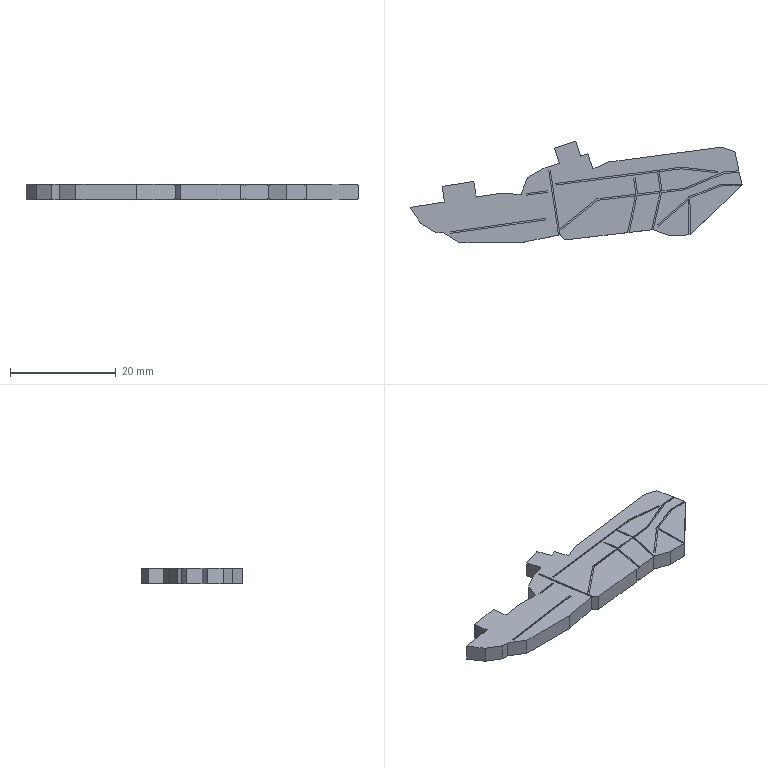Part | SolidWorks | features BaseBody 1 | 1 solid | 161 faces | box 62.766 x 19.221 x 3 mm | volume 2190 mm3 | plane 141 | spline 20